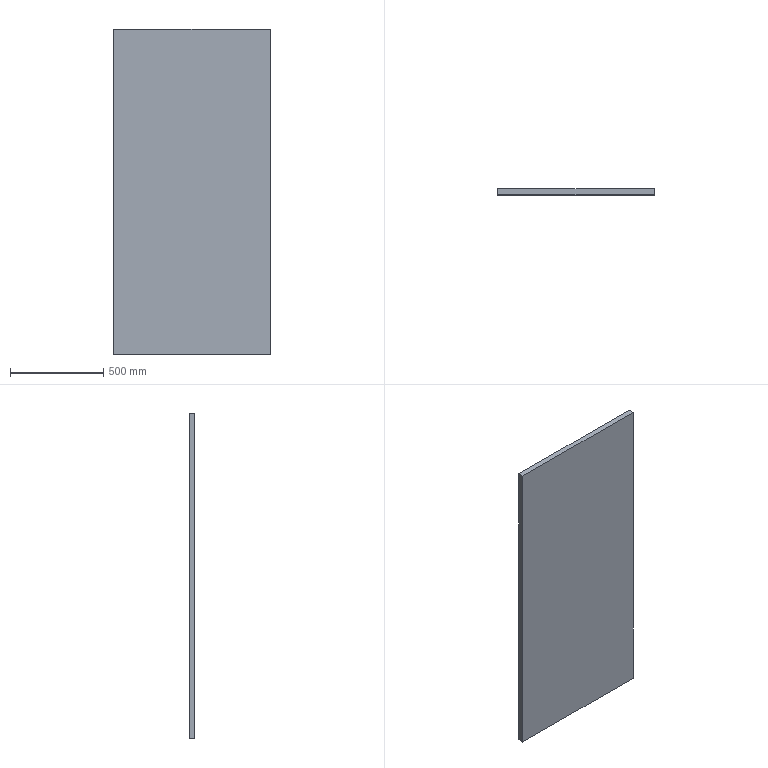Part | SolidWorks | features Extrusion 1 | 1 solid | 6 faces | box 840.28 x 30 x 1750 mm | volume 44114700 mm3 | plane 6
STEP:
#1=CARTESIAN_POINT('',(0.,0.,0.));
#2=VERTEX_POINT('',#1);
#3=CARTESIAN_POINT('',(0.,0.,1750.));
#4=VERTEX_POINT('',#3);
#5=CARTESIAN_POINT('',(0.,0.,1750.));
#6=DIRECTION('',(0.,0.,1.));
#7=VECTOR('',#6,1000.);
#8=LINE('',#5,#7);
#9=EDGE_CURVE('',#2,#4,#8,.T.);
#10=ORIENTED_EDGE('',*,*,#9,.T.);
#11=CARTESIAN_POINT('',(0.,30.,1750.));
#12=VERTEX_POINT('',#11);
#13=CARTESIAN_POINT('',(0.,30.,1750.));
#14=DIRECTION('',(0.,-1.,0.));
#15=VECTOR('',#14,1000.);
#16=LINE('',#13,#15);
#17=EDGE_CURVE('',#12,#4,#16,.T.);
#18=ORIENTED_EDGE('',*,*,#17,.F.);
#19=CARTESIAN_POINT('',(0.,30.,0.));
#20=VERTEX_POINT('',#19);
#21=CARTESIAN_POINT('',(0.,30.,1750.));
#22=DIRECTION('',(0.,0.,1.));
#23=VECTOR('',#22,1000.);
#24=LINE('',#21,#23);
#25=EDGE_CURVE('',#20,#12,#24,.T.);
#26=ORIENTED_EDGE('',*,*,#25,.F.);
#27=CARTESIAN_POINT('',(0.,30.,0.));
#28=DIRECTION('',(0.,-1.,0.));
#29=VECTOR('',#28,1000.);
#30=LINE('',#27,#29);
#31=EDGE_CURVE('',#20,#2,#30,.T.);
#32=ORIENTED_EDGE('',*,*,#31,.T.);
#33=EDGE_LOOP('',(#10,#18,#26,#32));
#34=FACE_OUTER_BOUND('',#33,.T.);
#35=CARTESIAN_POINT('',(0.,30.,1750.));
#36=DIRECTION('',(1.,0.,0.));
#37=DIRECTION('',(0.,0.,-1.));
#38=AXIS2_PLACEMENT_3D('',#35,#36,#37);
#39=PLANE('',#38);
#40=ADVANCED_FACE('',(#34),#39,.F.);
#41=CARTESIAN_POINT('',(840.28,0.,1750.));
#42=VERTEX_POINT('',#41);
#43=CARTESIAN_POINT('',(840.28,0.,1750.));
#44=DIRECTION('',(1.,0.,0.));
#45=VECTOR('',#44,1000.);
#46=LINE('',#43,#45);
#47=EDGE_CURVE('',#4,#42,#46,.T.);
#48=ORIENTED_EDGE('',*,*,#47,.T.);
#49=CARTESIAN_POINT('',(840.28,30.,1750.));
#50=VERTEX_POINT('',#49);
#51=CARTESIAN_POINT('',(840.28,30.,1750.));
#52=DIRECTION('',(0.,-1.,0.));
#53=VECTOR('',#52,1000.);
#54=LINE('',#51,#53);
#55=EDGE_CURVE('',#50,#42,#54,.T.);
#56=ORIENTED_EDGE('',*,*,#55,.F.);
#57=CARTESIAN_POINT('',(840.28,30.,1750.));
#58=DIRECTION('',(1.,0.,0.));
#59=VECTOR('',#58,1000.);
#60=LINE('',#57,#59);
#61=EDGE_CURVE('',#12,#50,#60,.T.);
#62=ORIENTED_EDGE('',*,*,#61,.F.);
#63=ORIENTED_EDGE('',*,*,#17,.T.);
#64=EDGE_LOOP('',(#48,#56,#62,#63));
#65=FACE_OUTER_BOUND('',#64,.T.);
#66=CARTESIAN_POINT('',(840.28,30.,1750.));
#67=DIRECTION('',(0.,0.,-1.));
#68=DIRECTION('',(-1.,0.,0.));
#69=AXIS2_PLACEMENT_3D('',#66,#67,#68);
#70=PLANE('',#69);
#71=ADVANCED_FACE('',(#65),#70,.F.);
#72=CARTESIAN_POINT('',(840.28,0.,0.));
#73=VERTEX_POINT('',#72);
#74=CARTESIAN_POINT('',(840.28,0.,0.));
#75=DIRECTION('',(0.,0.,-1.));
#76=VECTOR('',#75,1000.);
#77=LINE('',#74,#76);
#78=EDGE_CURVE('',#42,#73,#77,.T.);
#79=ORIENTED_EDGE('',*,*,#78,.T.);
#80=CARTESIAN_POINT('',(840.28,30.,0.));
#81=VERTEX_POINT('',#80);
#82=CARTESIAN_POINT('',(840.28,30.,0.));
#83=DIRECTION('',(0.,-1.,0.));
#84=VECTOR('',#83,1000.);
#85=LINE('',#82,#84);
#86=EDGE_CURVE('',#81,#73,#85,.T.);
#87=ORIENTED_EDGE('',*,*,#86,.F.);
#88=CARTESIAN_POINT('',(840.28,30.,0.));
#89=DIRECTION('',(0.,0.,-1.));
#90=VECTOR('',#89,1000.);
#91=LINE('',#88,#90);
#92=EDGE_CURVE('',#50,#81,#91,.T.);
#93=ORIENTED_EDGE('',*,*,#92,.F.);
#94=ORIENTED_EDGE('',*,*,#55,.T.);
#95=EDGE_LOOP('',(#79,#87,#93,#94));
#96=FACE_OUTER_BOUND('',#95,.T.);
#97=CARTESIAN_POINT('',(840.28,30.,0.));
#98=DIRECTION('',(-1.,0.,0.));
#99=DIRECTION('',(0.,0.,1.));
#100=AXIS2_PLACEMENT_3D('',#97,#98,#99);
#101=PLANE('',#100);
#102=ADVANCED_FACE('',(#96),#101,.F.);
#103=CARTESIAN_POINT('',(0.,0.,0.));
#104=DIRECTION('',(-1.,0.,0.));
#105=VECTOR('',#104,1000.);
#106=LINE('',#103,#105);
#107=EDGE_CURVE('',#73,#2,#106,.T.);
#108=ORIENTED_EDGE('',*,*,#107,.T.);
#109=ORIENTED_EDGE('',*,*,#31,.F.);
#110=CARTESIAN_POINT('',(0.,30.,0.));
#111=DIRECTION('',(-1.,0.,0.));
#112=VECTOR('',#111,1000.);
#113=LINE('',#110,#112);
#114=EDGE_CURVE('',#81,#20,#113,.T.);
#115=ORIENTED_EDGE('',*,*,#114,.F.);
#116=ORIENTED_EDGE('',*,*,#86,.T.);
#117=EDGE_LOOP('',(#108,#109,#115,#116));
#118=FACE_OUTER_BOUND('',#117,.T.);
#119=CARTESIAN_POINT('',(0.,30.,0.));
#120=DIRECTION('',(0.,0.,1.));
#121=DIRECTION('',(1.,0.,0.));
#122=AXIS2_PLACEMENT_3D('',#119,#120,#121);
#123=PLANE('',#122);
#124=ADVANCED_FACE('',(#118),#123,.F.);
#125=ORIENTED_EDGE('',*,*,#25,.T.);
#126=ORIENTED_EDGE('',*,*,#61,.T.);
#127=ORIENTED_EDGE('',*,*,#92,.T.);
#128=ORIENTED_EDGE('',*,*,#114,.T.);
#129=EDGE_LOOP('',(#125,#126,#127,#128));
#130=FACE_OUTER_BOUND('',#129,.T.);
#131=CARTESIAN_POINT('',(0.,30.,0.));
#132=DIRECTION('',(0.,-1.,0.));
#133=DIRECTION('',(0.,0.,-1.));
#134=AXIS2_PLACEMENT_3D('',#131,#132,#133);
#135=PLANE('',#134);
#136=ADVANCED_FACE('',(#130),#135,.F.);
#137=ORIENTED_EDGE('',*,*,#9,.F.);
#138=ORIENTED_EDGE('',*,*,#107,.F.);
#139=ORIENTED_EDGE('',*,*,#78,.F.);
#140=ORIENTED_EDGE('',*,*,#47,.F.);
#141=EDGE_LOOP('',(#137,#138,#139,#140));
#142=FACE_OUTER_BOUND('',#141,.T.);
#143=CARTESIAN_POINT('',(0.,0.,0.));
#144=DIRECTION('',(0.,-1.,0.));
#145=DIRECTION('',(0.,0.,-1.));
#146=AXIS2_PLACEMENT_3D('',#143,#144,#145);
#147=PLANE('',#146);
#148=ADVANCED_FACE('',(#142),#147,.T.);
#149=CLOSED_SHELL('',(#40,#71,#102,#124,#136,#148));
#150=MANIFOLD_SOLID_BREP('',#149);
#151=CARTESIAN_POINT('',(0.,0.,0.));
#152=DIRECTION('',(0.,0.,1.));
#153=DIRECTION('',(1.,0.,0.));
#154=AXIS2_PLACEMENT_3D('',#151,#152,#153);
#155=(LENGTH_UNIT()NAMED_UNIT(*)SI_UNIT(.MILLI.,.METRE.));
#156=UNCERTAINTY_MEASURE_WITH_UNIT(LENGTH_MEASURE(0.00001),#155,'','');
#157=(NAMED_UNIT(*)PLANE_ANGLE_UNIT()SI_UNIT($,.RADIAN.));
#158=(NAMED_UNIT(*)SI_UNIT($,.STERADIAN.)SOLID_ANGLE_UNIT());
#159=(GEOMETRIC_REPRESENTATION_CONTEXT(3)GLOBAL_UNCERTAINTY_ASSIGNED_CONTEXT((#156))GLOBAL_UNIT_ASSIGNED_CONTEXT((#155,#157,#158))REPRESENTATION_CONTEXT('',''));
#160=ADVANCED_BREP_SHAPE_REPRESENTATION('',(#150,#154),#159);